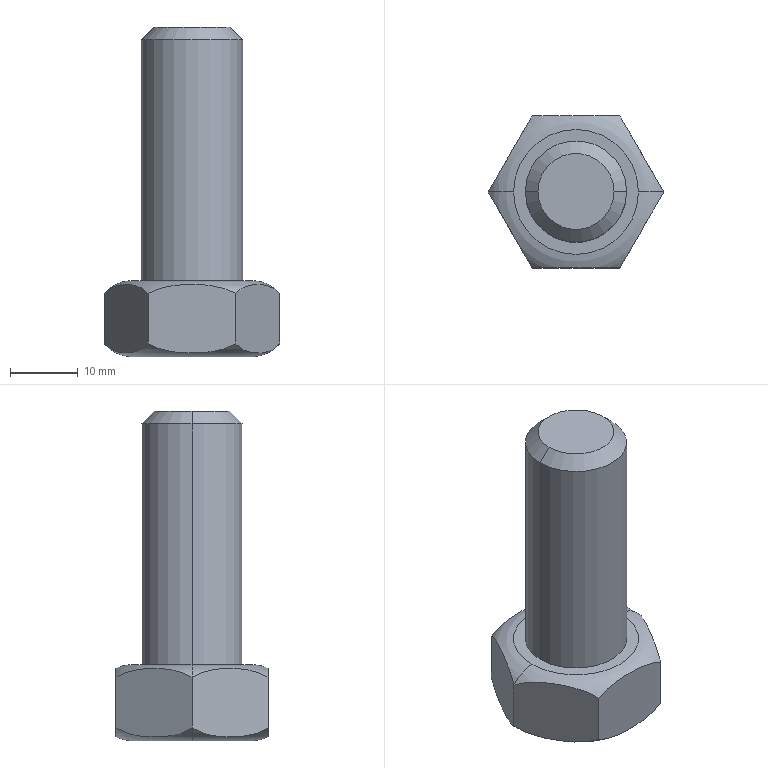Part | SolidWorks | features Chamfer 1, Extrusion 1, ICE 1, RevCut 1, Scale 1 | 1 solid | 17 faces | box 25.981 x 22.5 x 48.75 mm | volume 11356 mm3 | plane 9 | torus 4 | cone 2 | cylinder 2 | commonest cylinder face diameters 15 x2
STEP:
#1=CARTESIAN_POINT('',(9.24,0.00001748,-9.13));
#2=VERTEX_POINT('',#1);
#3=CARTESIAN_POINT('',(-9.24,0.00001748,-9.13));
#4=VERTEX_POINT('',#3);
#5=CARTESIAN_POINT('',(-0.000001168,0.00001748,-9.13));
#6=DIRECTION('',(0.,0.,1.));
#7=DIRECTION('',(1.,0.,0.));
#8=AXIS2_PLACEMENT_3D('',#5,#6,#7);
#9=CIRCLE('',#8,9.24);
#10=EDGE_CURVE('',#2,#4,#9,.T.);
#11=ORIENTED_EDGE('',*,*,#10,.T.);
#12=CARTESIAN_POINT('',(-12.99,0.00001748,-7.255));
#13=VERTEX_POINT('',#12);
#14=CARTESIAN_POINT('',(-8.781,0.00001748,-3.524));
#15=DIRECTION('',(0.,1.,0.));
#16=DIRECTION('',(-1.,0.,0.));
#17=AXIS2_PLACEMENT_3D('',#14,#15,#16);
#18=CIRCLE('',#17,5.625);
#19=EDGE_CURVE('',#4,#13,#18,.T.);
#20=ORIENTED_EDGE('',*,*,#19,.T.);
#21=CARTESIAN_POINT('',(-6.495,11.25,-7.255));
#22=VERTEX_POINT('',#21);
#23=CARTESIAN_POINT('',(-6.495,11.25,-7.255));
#24=CARTESIAN_POINT('',(-6.741,10.824,-7.533));
#25=CARTESIAN_POINT('',(-6.999,10.377,-7.746));
#26=CARTESIAN_POINT('',(-7.53,9.458,-8.089));
#27=CARTESIAN_POINT('',(-7.805,8.982,-8.217));
#28=CARTESIAN_POINT('',(-8.356,8.027,-8.41));
#29=CARTESIAN_POINT('',(-8.632,7.549,-8.474));
#30=CARTESIAN_POINT('',(-9.186,6.59,-8.558));
#31=CARTESIAN_POINT('',(-9.463,6.109,-8.578));
#32=CARTESIAN_POINT('',(-10.019,5.147,-8.578));
#33=CARTESIAN_POINT('',(-10.297,4.666,-8.559));
#34=CARTESIAN_POINT('',(-10.854,3.7,-8.474));
#35=CARTESIAN_POINT('',(-11.133,3.217,-8.409));
#36=CARTESIAN_POINT('',(-11.681,2.268,-8.217));
#37=CARTESIAN_POINT('',(-11.952,1.799,-8.091));
#38=CARTESIAN_POINT('',(-12.483,0.8793,-7.749));
#39=CARTESIAN_POINT('',(-12.745,0.4256,-7.532));
#40=CARTESIAN_POINT('',(-12.99,0.00001748,-7.255));
#41=B_SPLINE_CURVE_WITH_KNOTS('',3,(#23,#24,#25,#26,#27,#28,#29,#30,#31,#32,#33,#34,#35,#36,#37,#38,#39,#40),.UNSPECIFIED.,.F.,.F.,(4,2,2,2,2,2,2,2,4),(0.00000049,0.001672,0.003344,0.005016,0.006688,0.00836,0.01003,0.0117,0.01338),.UNSPECIFIED.);
#42=EDGE_CURVE('',#22,#13,#41,.T.);
#43=ORIENTED_EDGE('',*,*,#42,.F.);
#44=CARTESIAN_POINT('',(6.495,11.25,-7.255));
#45=VERTEX_POINT('',#44);
#46=CARTESIAN_POINT('',(6.495,11.25,-7.255));
#47=CARTESIAN_POINT('',(6.006,11.25,-7.531));
#48=CARTESIAN_POINT('',(5.491,11.25,-7.745));
#49=CARTESIAN_POINT('',(4.689,11.25,-8.004));
#50=CARTESIAN_POINT('',(4.417,11.25,-8.079));
#51=CARTESIAN_POINT('',(3.871,11.25,-8.21));
#52=CARTESIAN_POINT('',(3.597,11.25,-8.266));
#53=CARTESIAN_POINT('',(2.772,11.25,-8.41));
#54=CARTESIAN_POINT('',(2.218,11.25,-8.475));
#55=CARTESIAN_POINT('',(1.106,11.25,-8.559));
#56=CARTESIAN_POINT('',(0.5448,11.25,-8.579));
#57=CARTESIAN_POINT('',(-0.5739,11.25,-8.578));
#58=CARTESIAN_POINT('',(-1.13,11.25,-8.558));
#59=CARTESIAN_POINT('',(-2.235,11.25,-8.473));
#60=CARTESIAN_POINT('',(-2.784,11.25,-8.408));
#61=CARTESIAN_POINT('',(-3.872,11.25,-8.218));
#62=CARTESIAN_POINT('',(-4.412,11.25,-8.092));
#63=CARTESIAN_POINT('',(-5.476,11.25,-7.751));
#64=CARTESIAN_POINT('',(-6.004,11.25,-7.532));
#65=CARTESIAN_POINT('',(-6.495,11.25,-7.255));
#66=B_SPLINE_CURVE_WITH_KNOTS('',3,(#46,#47,#48,#49,#50,#51,#52,#53,#54,#55,#56,#57,#58,#59,#60,#61,#62,#63,#64,#65),.UNSPECIFIED.,.F.,.F.,(4,2,2,2,2,2,2,2,2,4),(0.03832,0.03997,0.0408,0.04163,0.04329,0.04495,0.0466,0.04826,0.04992,0.05157),.UNSPECIFIED.);
#67=EDGE_CURVE('',#45,#22,#66,.T.);
#68=ORIENTED_EDGE('',*,*,#67,.F.);
#69=CARTESIAN_POINT('',(12.99,0.00001748,-7.255));
#70=VERTEX_POINT('',#69);
#71=CARTESIAN_POINT('',(12.99,0.00001748,-7.255));
#72=CARTESIAN_POINT('',(12.744,0.4264,-7.533));
#73=CARTESIAN_POINT('',(12.486,0.8728,-7.746));
#74=CARTESIAN_POINT('',(11.956,1.792,-8.089));
#75=CARTESIAN_POINT('',(11.681,2.268,-8.217));
#76=CARTESIAN_POINT('',(11.13,3.223,-8.41));
#77=CARTESIAN_POINT('',(10.853,3.701,-8.474));
#78=CARTESIAN_POINT('',(10.3,4.66,-8.558));
#79=CARTESIAN_POINT('',(10.022,5.141,-8.578));
#80=CARTESIAN_POINT('',(9.467,6.103,-8.578));
#81=CARTESIAN_POINT('',(9.189,6.585,-8.559));
#82=CARTESIAN_POINT('',(8.631,7.55,-8.474));
#83=CARTESIAN_POINT('',(8.353,8.033,-8.409));
#84=CARTESIAN_POINT('',(7.804,8.982,-8.217));
#85=CARTESIAN_POINT('',(7.534,9.451,-8.091));
#86=CARTESIAN_POINT('',(7.003,10.371,-7.749));
#87=CARTESIAN_POINT('',(6.741,10.824,-7.532));
#88=CARTESIAN_POINT('',(6.495,11.25,-7.255));
#89=B_SPLINE_CURVE_WITH_KNOTS('',3,(#71,#72,#73,#74,#75,#76,#77,#78,#79,#80,#81,#82,#83,#84,#85,#86,#87,#88),.UNSPECIFIED.,.F.,.F.,(4,2,2,2,2,2,2,2,4),(0.00000049,0.001672,0.003344,0.005016,0.006688,0.00836,0.01003,0.0117,0.01338),.UNSPECIFIED.);
#90=EDGE_CURVE('',#70,#45,#89,.T.);
#91=ORIENTED_EDGE('',*,*,#90,.F.);
#92=CARTESIAN_POINT('',(8.781,0.00001748,-3.524));
#93=DIRECTION('',(0.,-1.,0.));
#94=DIRECTION('',(0.,0.,-1.));
#95=AXIS2_PLACEMENT_3D('',#92,#93,#94);
#96=CIRCLE('',#95,5.625);
#97=EDGE_CURVE('',#2,#70,#96,.T.);
#98=ORIENTED_EDGE('',*,*,#97,.F.);
#99=EDGE_LOOP('',(#11,#20,#43,#68,#91,#98));
#100=FACE_OUTER_BOUND('',#99,.T.);
#101=CARTESIAN_POINT('',(-0.000001168,0.00001748,-3.524));
#102=DIRECTION('',(0.,0.,1.));
#103=DIRECTION('',(1.,0.,0.));
#104=AXIS2_PLACEMENT_3D('',#101,#102,#103);
#105=TOROIDAL_SURFACE('',#104,8.781,5.625);
#106=ADVANCED_FACE('',(#100),#105,.T.);
#107=CARTESIAN_POINT('',(-12.99,0.00001748,0.2448));
#108=VERTEX_POINT('',#107);
#109=CARTESIAN_POINT('',(-6.495,11.25,0.2448));
#110=VERTEX_POINT('',#109);
#111=CARTESIAN_POINT('',(-12.99,0.00001748,0.2448));
#112=CARTESIAN_POINT('',(-12.744,0.4264,0.5225));
#113=CARTESIAN_POINT('',(-12.486,0.8728,0.736));
#114=CARTESIAN_POINT('',(-11.956,1.792,1.078));
#115=CARTESIAN_POINT('',(-11.681,2.268,1.207));
#116=CARTESIAN_POINT('',(-11.13,3.223,1.399));
#117=CARTESIAN_POINT('',(-10.853,3.701,1.464));
#118=CARTESIAN_POINT('',(-10.3,4.66,1.548));
#119=CARTESIAN_POINT('',(-10.022,5.141,1.568));
#120=CARTESIAN_POINT('',(-9.467,6.103,1.568));
#121=CARTESIAN_POINT('',(-9.189,6.585,1.548));
#122=CARTESIAN_POINT('',(-8.631,7.55,1.464));
#123=CARTESIAN_POINT('',(-8.353,8.033,1.398));
#124=CARTESIAN_POINT('',(-7.804,8.982,1.206));
#125=CARTESIAN_POINT('',(-7.534,9.451,1.08));
#126=CARTESIAN_POINT('',(-7.003,10.371,0.7389));
#127=CARTESIAN_POINT('',(-6.741,10.824,0.5219));
#128=CARTESIAN_POINT('',(-6.495,11.25,0.2448));
#129=B_SPLINE_CURVE_WITH_KNOTS('',3,(#111,#112,#113,#114,#115,#116,#117,#118,#119,#120,#121,#122,#123,#124,#125,#126,#127,#128),.UNSPECIFIED.,.F.,.F.,(4,2,2,2,2,2,2,2,4),(0.00000049,0.001672,0.003344,0.005016,0.006688,0.00836,0.01003,0.0117,0.01338),.UNSPECIFIED.);
#130=EDGE_CURVE('',#108,#110,#129,.T.);
#131=ORIENTED_EDGE('',*,*,#130,.F.);
#132=CARTESIAN_POINT('',(-9.24,0.00001748,2.12));
#133=VERTEX_POINT('',#132);
#134=CARTESIAN_POINT('',(-8.781,0.00001748,-3.486));
#135=DIRECTION('',(0.,1.,0.));
#136=DIRECTION('',(-1.,0.,0.));
#137=AXIS2_PLACEMENT_3D('',#134,#135,#136);
#138=CIRCLE('',#137,5.625);
#139=EDGE_CURVE('',#108,#133,#138,.T.);
#140=ORIENTED_EDGE('',*,*,#139,.T.);
#141=CARTESIAN_POINT('',(9.24,0.00001748,2.12));
#142=VERTEX_POINT('',#141);
#143=CARTESIAN_POINT('',(-0.000001168,0.00001748,2.12));
#144=DIRECTION('',(0.,0.,1.));
#145=DIRECTION('',(1.,0.,0.));
#146=AXIS2_PLACEMENT_3D('',#143,#144,#145);
#147=CIRCLE('',#146,9.24);
#148=EDGE_CURVE('',#142,#133,#147,.T.);
#149=ORIENTED_EDGE('',*,*,#148,.F.);
#150=CARTESIAN_POINT('',(12.99,0.00001748,0.2448));
#151=VERTEX_POINT('',#150);
#152=CARTESIAN_POINT('',(8.781,0.00001748,-3.486));
#153=DIRECTION('',(0.,-1.,0.));
#154=DIRECTION('',(0.,0.,-1.));
#155=AXIS2_PLACEMENT_3D('',#152,#153,#154);
#156=CIRCLE('',#155,5.625);
#157=EDGE_CURVE('',#151,#142,#156,.T.);
#158=ORIENTED_EDGE('',*,*,#157,.F.);
#159=CARTESIAN_POINT('',(6.495,11.25,0.2448));
#160=VERTEX_POINT('',#159);
#161=CARTESIAN_POINT('',(6.495,11.25,0.2448));
#162=CARTESIAN_POINT('',(6.741,10.824,0.5225));
#163=CARTESIAN_POINT('',(6.999,10.377,0.736));
#164=CARTESIAN_POINT('',(7.53,9.458,1.078));
#165=CARTESIAN_POINT('',(7.805,8.982,1.207));
#166=CARTESIAN_POINT('',(8.356,8.027,1.399));
#167=CARTESIAN_POINT('',(8.632,7.549,1.464));
#168=CARTESIAN_POINT('',(9.186,6.59,1.548));
#169=CARTESIAN_POINT('',(9.463,6.109,1.568));
#170=CARTESIAN_POINT('',(10.019,5.147,1.568));
#171=CARTESIAN_POINT('',(10.297,4.666,1.548));
#172=CARTESIAN_POINT('',(10.854,3.7,1.464));
#173=CARTESIAN_POINT('',(11.133,3.217,1.398));
#174=CARTESIAN_POINT('',(11.681,2.268,1.206));
#175=CARTESIAN_POINT('',(11.952,1.799,1.08));
#176=CARTESIAN_POINT('',(12.483,0.8793,0.7389));
#177=CARTESIAN_POINT('',(12.745,0.4256,0.5219));
#178=CARTESIAN_POINT('',(12.99,0.00001748,0.2448));
#179=B_SPLINE_CURVE_WITH_KNOTS('',3,(#161,#162,#163,#164,#165,#166,#167,#168,#169,#170,#171,#172,#173,#174,#175,#176,#177,#178),.UNSPECIFIED.,.F.,.F.,(4,2,2,2,2,2,2,2,4),(0.00000049,0.001672,0.003344,0.005016,0.006688,0.00836,0.01003,0.0117,0.01338),.UNSPECIFIED.);
#180=EDGE_CURVE('',#160,#151,#179,.T.);
#181=ORIENTED_EDGE('',*,*,#180,.F.);
#182=CARTESIAN_POINT('',(-6.495,11.25,0.2448));
#183=CARTESIAN_POINT('',(-6.006,11.25,0.5206));
#184=CARTESIAN_POINT('',(-5.491,11.25,0.735));
#185=CARTESIAN_POINT('',(-4.689,11.25,0.9932));
#186=CARTESIAN_POINT('',(-4.417,11.25,1.069));
#187=CARTESIAN_POINT('',(-3.871,11.25,1.2));
#188=CARTESIAN_POINT('',(-3.597,11.25,1.255));
#189=CARTESIAN_POINT('',(-2.772,11.25,1.399));
#190=CARTESIAN_POINT('',(-2.218,11.25,1.464));
#191=CARTESIAN_POINT('',(-1.106,11.25,1.548));
#192=CARTESIAN_POINT('',(-0.5448,11.25,1.568));
#193=CARTESIAN_POINT('',(0.5739,11.25,1.567));
#194=CARTESIAN_POINT('',(1.13,11.25,1.547));
#195=CARTESIAN_POINT('',(2.235,11.25,1.462));
#196=CARTESIAN_POINT('',(2.784,11.25,1.397));
#197=CARTESIAN_POINT('',(3.872,11.25,1.207));
#198=CARTESIAN_POINT('',(4.412,11.25,1.082));
#199=CARTESIAN_POINT('',(5.476,11.25,0.7405));
#200=CARTESIAN_POINT('',(6.004,11.25,0.5218));
#201=CARTESIAN_POINT('',(6.495,11.25,0.2448));
#202=B_SPLINE_CURVE_WITH_KNOTS('',3,(#182,#183,#184,#185,#186,#187,#188,#189,#190,#191,#192,#193,#194,#195,#196,#197,#198,#199,#200,#201),.UNSPECIFIED.,.F.,.F.,(4,2,2,2,2,2,2,2,2,4),(0.03832,0.03997,0.0408,0.04163,0.04329,0.04495,0.0466,0.04826,0.04992,0.05157),.UNSPECIFIED.);
#203=EDGE_CURVE('',#110,#160,#202,.T.);
#204=ORIENTED_EDGE('',*,*,#203,.F.);
#205=EDGE_LOOP('',(#131,#140,#149,#158,#181,#204));
#206=FACE_OUTER_BOUND('',#205,.T.);
#207=CARTESIAN_POINT('',(-0.000001168,0.00001748,-3.486));
#208=DIRECTION('',(0.,0.,1.));
#209=DIRECTION('',(1.,0.,0.));
#210=AXIS2_PLACEMENT_3D('',#207,#208,#209);
#211=TOROIDAL_SURFACE('',#210,8.781,5.625);
#212=ADVANCED_FACE('',(#206),#211,.T.);
#213=CARTESIAN_POINT('',(5.625,0.00001748,39.62));
#214=VERTEX_POINT('',#213);
#215=CARTESIAN_POINT('',(-5.625,0.00001748,39.62));
#216=VERTEX_POINT('',#215);
#217=CARTESIAN_POINT('',(-0.000001168,0.00001748,39.62));
#218=DIRECTION('',(0.,0.,1.));
#219=DIRECTION('',(1.,0.,0.));
#220=AXIS2_PLACEMENT_3D('',#217,#218,#219);
#221=CIRCLE('',#220,5.625);
#222=EDGE_CURVE('',#214,#216,#221,.T.);
#223=ORIENTED_EDGE('',*,*,#222,.F.);
#224=CARTESIAN_POINT('',(7.5,0.00001748,37.745));
#225=VERTEX_POINT('',#224);
#226=CARTESIAN_POINT('',(5.625,0.00001748,39.62));
#227=DIRECTION('',(0.7071,0.,-0.7071));
#228=VECTOR('',#227,1000.);
#229=LINE('',#226,#228);
#230=EDGE_CURVE('',#214,#225,#229,.T.);
#231=ORIENTED_EDGE('',*,*,#230,.T.);
#232=CARTESIAN_POINT('',(-7.5,0.00001748,37.745));
#233=VERTEX_POINT('',#232);
#234=CARTESIAN_POINT('',(-0.000001168,0.00001748,37.745));
#235=DIRECTION('',(0.,0.,-1.));
#236=DIRECTION('',(1.,0.,0.));
#237=AXIS2_PLACEMENT_3D('',#234,#235,#236);
#238=CIRCLE('',#237,7.5);
#239=EDGE_CURVE('',#233,#225,#238,.T.);
#240=ORIENTED_EDGE('',*,*,#239,.F.);
#241=CARTESIAN_POINT('',(-5.625,0.00001748,39.62));
#242=DIRECTION('',(-0.7071,0.,-0.7071));
#243=VECTOR('',#242,1000.);
#244=LINE('',#241,#243);
#245=EDGE_CURVE('',#216,#233,#244,.T.);
#246=ORIENTED_EDGE('',*,*,#245,.F.);
#247=EDGE_LOOP('',(#223,#231,#240,#246));
#248=FACE_OUTER_BOUND('',#247,.T.);
#249=CARTESIAN_POINT('',(-0.000001168,0.00001748,39.62));
#250=DIRECTION('',(0.,0.,-1.));
#251=DIRECTION('',(-1.,0.,0.));
#252=AXIS2_PLACEMENT_3D('',#249,#250,#251);
#253=CONICAL_SURFACE('',#252,5.625,0.7854);
#254=ADVANCED_FACE('',(#248),#253,.T.);
#255=ORIENTED_EDGE('',*,*,#239,.T.);
#256=CARTESIAN_POINT('',(7.5,0.00001748,2.12));
#257=VERTEX_POINT('',#256);
#258=CARTESIAN_POINT('',(7.5,0.00001748,39.62));
#259=DIRECTION('',(0.,0.,-1.));
#260=VECTOR('',#259,1000.);
#261=LINE('',#258,#260);
#262=EDGE_CURVE('',#225,#257,#261,.T.);
#263=ORIENTED_EDGE('',*,*,#262,.T.);
#264=CARTESIAN_POINT('',(-7.5,0.00001748,2.12));
#265=VERTEX_POINT('',#264);
#266=CARTESIAN_POINT('',(-0.000001168,0.00001748,2.12));
#267=DIRECTION('',(0.,0.,1.));
#268=DIRECTION('',(1.,0.,0.));
#269=AXIS2_PLACEMENT_3D('',#266,#267,#268);
#270=CIRCLE('',#269,7.5);
#271=EDGE_CURVE('',#257,#265,#270,.T.);
#272=ORIENTED_EDGE('',*,*,#271,.T.);
#273=CARTESIAN_POINT('',(-7.5,0.00001748,39.62));
#274=DIRECTION('',(0.,0.,-1.));
#275=VECTOR('',#274,1000.);
#276=LINE('',#273,#275);
#277=EDGE_CURVE('',#233,#265,#276,.T.);
#278=ORIENTED_EDGE('',*,*,#277,.F.);
#279=EDGE_LOOP('',(#255,#263,#272,#278));
#280=FACE_OUTER_BOUND('',#279,.T.);
#281=CARTESIAN_POINT('',(-0.000001168,0.00001748,39.62));
#282=DIRECTION('',(0.,0.,-1.));
#283=DIRECTION('',(-1.,0.,0.));
#284=AXIS2_PLACEMENT_3D('',#281,#282,#283);
#285=CYLINDRICAL_SURFACE('',#284,7.5);
#286=ADVANCED_FACE('',(#280),#285,.T.);
#287=CARTESIAN_POINT('',(-0.000001168,0.00001748,2.12));
#288=DIRECTION('',(0.,0.,1.));
#289=DIRECTION('',(1.,0.,0.));
#290=AXIS2_PLACEMENT_3D('',#287,#288,#289);
#291=CIRCLE('',#290,7.5);
#292=EDGE_CURVE('',#265,#257,#291,.T.);
#293=ORIENTED_EDGE('',*,*,#292,.F.);
#294=ORIENTED_EDGE('',*,*,#271,.F.);
#295=EDGE_LOOP('',(#293,#294));
#296=FACE_BOUND('',#295,.T.);
#297=ORIENTED_EDGE('',*,*,#148,.T.);
#298=CARTESIAN_POINT('',(-0.000001168,0.00001748,2.12));
#299=DIRECTION('',(0.,0.,1.));
#300=DIRECTION('',(1.,0.,0.));
#301=AXIS2_PLACEMENT_3D('',#298,#299,#300);
#302=CIRCLE('',#301,9.24);
#303=EDGE_CURVE('',#133,#142,#302,.T.);
#304=ORIENTED_EDGE('',*,*,#303,.T.);
#305=EDGE_LOOP('',(#297,#304));
#306=FACE_OUTER_BOUND('',#305,.T.);
#307=CARTESIAN_POINT('',(-0.000001168,0.00001748,2.12));
#308=DIRECTION('',(0.,0.,1.));
#309=DIRECTION('',(1.,0.,0.));
#310=AXIS2_PLACEMENT_3D('',#307,#308,#309);
#311=PLANE('',#310);
#312=ADVANCED_FACE('',(#296,#306),#311,.T.);
#313=ORIENTED_EDGE('',*,*,#262,.F.);
#314=CARTESIAN_POINT('',(-0.000001168,0.00001748,37.745));
#315=DIRECTION('',(0.,0.,-1.));
#316=DIRECTION('',(1.,0.,0.));
#317=AXIS2_PLACEMENT_3D('',#314,#315,#316);
#318=CIRCLE('',#317,7.5);
#319=EDGE_CURVE('',#225,#233,#318,.T.);
#320=ORIENTED_EDGE('',*,*,#319,.T.);
#321=ORIENTED_EDGE('',*,*,#277,.T.);
#322=ORIENTED_EDGE('',*,*,#292,.T.);
#323=EDGE_LOOP('',(#313,#320,#321,#322));
#324=FACE_OUTER_BOUND('',#323,.T.);
#325=CARTESIAN_POINT('',(-0.000001168,0.00001748,39.62));
#326=DIRECTION('',(0.,0.,-1.));
#327=DIRECTION('',(-1.,0.,0.));
#328=AXIS2_PLACEMENT_3D('',#325,#326,#327);
#329=CYLINDRICAL_SURFACE('',#328,7.5);
#330=ADVANCED_FACE('',(#324),#329,.T.);
#331=CARTESIAN_POINT('',(-0.000001168,0.00001748,39.62));
#332=DIRECTION('',(0.,0.,1.));
#333=DIRECTION('',(1.,0.,0.));
#334=AXIS2_PLACEMENT_3D('',#331,#332,#333);
#335=CIRCLE('',#334,5.625);
#336=EDGE_CURVE('',#216,#214,#335,.T.);
#337=ORIENTED_EDGE('',*,*,#336,.T.);
#338=ORIENTED_EDGE('',*,*,#222,.T.);
#339=EDGE_LOOP('',(#337,#338));
#340=FACE_OUTER_BOUND('',#339,.T.);
#341=CARTESIAN_POINT('',(-0.000001168,0.00001748,39.62));
#342=DIRECTION('',(0.,0.,1.));
#343=DIRECTION('',(1.,0.,0.));
#344=AXIS2_PLACEMENT_3D('',#341,#342,#343);
#345=PLANE('',#344);
#346=ADVANCED_FACE('',(#340),#345,.T.);
#347=ORIENTED_EDGE('',*,*,#230,.F.);
#348=ORIENTED_EDGE('',*,*,#336,.F.);
#349=ORIENTED_EDGE('',*,*,#245,.T.);
#350=ORIENTED_EDGE('',*,*,#319,.F.);
#351=EDGE_LOOP('',(#347,#348,#349,#350));
#352=FACE_OUTER_BOUND('',#351,.T.);
#353=CARTESIAN_POINT('',(-0.000001168,0.00001748,39.62));
#354=DIRECTION('',(0.,0.,-1.));
#355=DIRECTION('',(-1.,0.,0.));
#356=AXIS2_PLACEMENT_3D('',#353,#354,#355);
#357=CONICAL_SURFACE('',#356,5.625,0.7854);
#358=ADVANCED_FACE('',(#352),#357,.T.);
#359=ORIENTED_EDGE('',*,*,#139,.F.);
#360=CARTESIAN_POINT('',(-6.495,-11.25,0.2448));
#361=VERTEX_POINT('',#360);
#362=CARTESIAN_POINT('',(-6.495,-11.25,0.2448));
#363=CARTESIAN_POINT('',(-6.741,-10.824,0.5225));
#364=CARTESIAN_POINT('',(-6.999,-10.377,0.736));
#365=CARTESIAN_POINT('',(-7.53,-9.458,1.078));
#366=CARTESIAN_POINT('',(-7.805,-8.982,1.207));
#367=CARTESIAN_POINT('',(-8.356,-8.027,1.399));
#368=CARTESIAN_POINT('',(-8.632,-7.549,1.464));
#369=CARTESIAN_POINT('',(-9.186,-6.59,1.548));
#370=CARTESIAN_POINT('',(-9.463,-6.109,1.568));
#371=CARTESIAN_POINT('',(-10.019,-5.147,1.568));
#372=CARTESIAN_POINT('',(-10.297,-4.665,1.548));
#373=CARTESIAN_POINT('',(-10.854,-3.7,1.464));
#374=CARTESIAN_POINT('',(-11.133,-3.217,1.398));
#375=CARTESIAN_POINT('',(-11.681,-2.268,1.206));
#376=CARTESIAN_POINT('',(-11.952,-1.799,1.08));
#377=CARTESIAN_POINT('',(-12.483,-0.8793,0.7389));
#378=CARTESIAN_POINT('',(-12.745,-0.4255,0.5219));
#379=CARTESIAN_POINT('',(-12.99,0.00001748,0.2448));
#380=B_SPLINE_CURVE_WITH_KNOTS('',3,(#362,#363,#364,#365,#366,#367,#368,#369,#370,#371,#372,#373,#374,#375,#376,#377,#378,#379),.UNSPECIFIED.,.F.,.F.,(4,2,2,2,2,2,2,2,4),(0.00000049,0.001672,0.003344,0.005016,0.006688,0.00836,0.01003,0.0117,0.01338),.UNSPECIFIED.);
#381=EDGE_CURVE('',#361,#108,#380,.T.);
#382=ORIENTED_EDGE('',*,*,#381,.F.);
#383=CARTESIAN_POINT('',(6.495,-11.25,0.2448));
#384=VERTEX_POINT('',#383);
#385=CARTESIAN_POINT('',(6.495,-11.25,0.2448));
#386=CARTESIAN_POINT('',(6.006,-11.25,0.5206));
#387=CARTESIAN_POINT('',(5.491,-11.25,0.735));
#388=CARTESIAN_POINT('',(4.689,-11.25,0.9932));
#389=CARTESIAN_POINT('',(4.417,-11.25,1.069));
#390=CARTESIAN_POINT('',(3.871,-11.25,1.2));
#391=CARTESIAN_POINT('',(3.597,-11.25,1.255));
#392=CARTESIAN_POINT('',(2.772,-11.25,1.399));
#393=CARTESIAN_POINT('',(2.218,-11.25,1.464));
#394=CARTESIAN_POINT('',(1.106,-11.25,1.548));
#395=CARTESIAN_POINT('',(0.5448,-11.25,1.568));
#396=CARTESIAN_POINT('',(-0.5739,-11.25,1.567));
#397=CARTESIAN_POINT('',(-1.13,-11.25,1.547));
#398=CARTESIAN_POINT('',(-2.235,-11.25,1.462));
#399=CARTESIAN_POINT('',(-2.784,-11.25,1.397));
#400=CARTESIAN_POINT('',(-3.872,-11.25,1.207));
#401=CARTESIAN_POINT('',(-4.412,-11.25,1.082));
#402=CARTESIAN_POINT('',(-5.476,-11.25,0.7405));
#403=CARTESIAN_POINT('',(-6.004,-11.25,0.5218));
#404=CARTESIAN_POINT('',(-6.495,-11.25,0.2448));
#405=B_SPLINE_CURVE_WITH_KNOTS('',3,(#385,#386,#387,#388,#389,#390,#391,#392,#393,#394,#395,#396,#397,#398,#399,#400,#401,#402,#403,#404),.UNSPECIFIED.,.F.,.F.,(4,2,2,2,2,2,2,2,2,4),(0.03832,0.03997,0.0408,0.04163,0.04329,0.04495,0.0466,0.04826,0.04992,0.05157),.UNSPECIFIED.);
#406=EDGE_CURVE('',#384,#361,#405,.T.);
#407=ORIENTED_EDGE('',*,*,#406,.F.);
#408=CARTESIAN_POINT('',(12.99,0.00001748,0.2448));
#409=CARTESIAN_POINT('',(12.744,-0.4264,0.5225));
#410=CARTESIAN_POINT('',(12.486,-0.8728,0.736));
#411=CARTESIAN_POINT('',(11.956,-1.792,1.078));
#412=CARTESIAN_POINT('',(11.681,-2.268,1.207));
#413=CARTESIAN_POINT('',(11.13,-3.223,1.399));
#414=CARTESIAN_POINT('',(10.853,-3.701,1.464));
#415=CARTESIAN_POINT('',(10.3,-4.66,1.548));
#416=CARTESIAN_POINT('',(10.022,-5.141,1.568));
#417=CARTESIAN_POINT('',(9.467,-6.103,1.568));
#418=CARTESIAN_POINT('',(9.189,-6.584,1.548));
#419=CARTESIAN_POINT('',(8.631,-7.55,1.464));
#420=CARTESIAN_POINT('',(8.353,-8.033,1.398));
#421=CARTESIAN_POINT('',(7.804,-8.982,1.206));
#422=CARTESIAN_POINT('',(7.534,-9.451,1.08));
#423=CARTESIAN_POINT('',(7.003,-10.371,0.7389));
#424=CARTESIAN_POINT('',(6.741,-10.824,0.5219));
#425=CARTESIAN_POINT('',(6.495,-11.25,0.2448));
#426=B_SPLINE_CURVE_WITH_KNOTS('',3,(#408,#409,#410,#411,#412,#413,#414,#415,#416,#417,#418,#419,#420,#421,#422,#423,#424,#425),.UNSPECIFIED.,.F.,.F.,(4,2,2,2,2,2,2,2,4),(0.00000049,0.001672,0.003344,0.005016,0.006688,0.00836,0.01003,0.0117,0.01338),.UNSPECIFIED.);
#427=EDGE_CURVE('',#151,#384,#426,.T.);
#428=ORIENTED_EDGE('',*,*,#427,.F.);
#429=ORIENTED_EDGE('',*,*,#157,.T.);
#430=ORIENTED_EDGE('',*,*,#303,.F.);
#431=EDGE_LOOP('',(#359,#382,#407,#428,#429,#430));
#432=FACE_OUTER_BOUND('',#431,.T.);
#433=CARTESIAN_POINT('',(-0.000001168,0.00001748,-3.486));
#434=DIRECTION('',(0.,0.,1.));
#435=DIRECTION('',(1.,0.,0.));
#436=AXIS2_PLACEMENT_3D('',#433,#434,#435);
#437=TOROIDAL_SURFACE('',#436,8.781,5.625);
#438=ADVANCED_FACE('',(#432),#437,.T.);
#439=ORIENTED_EDGE('',*,*,#10,.F.);
#440=CARTESIAN_POINT('',(-0.000001168,0.00001748,-9.13));
#441=DIRECTION('',(0.,0.,1.));
#442=DIRECTION('',(1.,0.,0.));
#443=AXIS2_PLACEMENT_3D('',#440,#441,#442);
#444=CIRCLE('',#443,9.24);
#445=EDGE_CURVE('',#4,#2,#444,.T.);
#446=ORIENTED_EDGE('',*,*,#445,.F.);
#447=EDGE_LOOP('',(#439,#446));
#448=FACE_OUTER_BOUND('',#447,.T.);
#449=CARTESIAN_POINT('',(-0.000001168,0.00001748,-9.13));
#450=DIRECTION('',(0.,0.,1.));
#451=DIRECTION('',(1.,0.,0.));
#452=AXIS2_PLACEMENT_3D('',#449,#450,#451);
#453=PLANE('',#452);
#454=ADVANCED_FACE('',(#448),#453,.F.);
#455=ORIENTED_EDGE('',*,*,#19,.F.);
#456=ORIENTED_EDGE('',*,*,#445,.T.);
#457=ORIENTED_EDGE('',*,*,#97,.T.);
#458=CARTESIAN_POINT('',(6.495,-11.25,-7.255));
#459=VERTEX_POINT('',#458);
#460=CARTESIAN_POINT('',(6.495,-11.25,-7.255));
#461=CARTESIAN_POINT('',(6.741,-10.824,-7.533));
#462=CARTESIAN_POINT('',(6.999,-10.377,-7.746));
#463=CARTESIAN_POINT('',(7.53,-9.458,-8.089));
#464=CARTESIAN_POINT('',(7.805,-8.982,-8.217));
#465=CARTESIAN_POINT('',(8.356,-8.027,-8.41));
#466=CARTESIAN_POINT('',(8.632,-7.549,-8.474));
#467=CARTESIAN_POINT('',(9.186,-6.59,-8.558));
#468=CARTESIAN_POINT('',(9.463,-6.109,-8.578));
#469=CARTESIAN_POINT('',(10.019,-5.147,-8.578));
#470=CARTESIAN_POINT('',(10.297,-4.665,-8.559));
#471=CARTESIAN_POINT('',(10.854,-3.7,-8.474));
#472=CARTESIAN_POINT('',(11.133,-3.217,-8.409));
#473=CARTESIAN_POINT('',(11.681,-2.268,-8.217));
#474=CARTESIAN_POINT('',(11.952,-1.799,-8.091));
#475=CARTESIAN_POINT('',(12.483,-0.8793,-7.749));
#476=CARTESIAN_POINT('',(12.745,-0.4255,-7.532));
#477=CARTESIAN_POINT('',(12.99,0.00001748,-7.255));
#478=B_SPLINE_CURVE_WITH_KNOTS('',3,(#460,#461,#462,#463,#464,#465,#466,#467,#468,#469,#470,#471,#472,#473,#474,#475,#476,#477),.UNSPECIFIED.,.F.,.F.,(4,2,2,2,2,2,2,2,4),(0.00000049,0.001672,0.003344,0.005016,0.006688,0.00836,0.01003,0.0117,0.01338),.UNSPECIFIED.);
#479=EDGE_CURVE('',#459,#70,#478,.T.);
#480=ORIENTED_EDGE('',*,*,#479,.F.);
#481=CARTESIAN_POINT('',(-6.495,-11.25,-7.255));
#482=VERTEX_POINT('',#481);
#483=CARTESIAN_POINT('',(-6.495,-11.25,-7.255));
#484=CARTESIAN_POINT('',(-6.006,-11.25,-7.531));
#485=CARTESIAN_POINT('',(-5.491,-11.25,-7.745));
#486=CARTESIAN_POINT('',(-4.689,-11.25,-8.004));
#487=CARTESIAN_POINT('',(-4.417,-11.25,-8.079));
#488=CARTESIAN_POINT('',(-3.871,-11.25,-8.21));
#489=CARTESIAN_POINT('',(-3.597,-11.25,-8.266));
#490=CARTESIAN_POINT('',(-2.772,-11.25,-8.41));
#491=CARTESIAN_POINT('',(-2.218,-11.25,-8.475));
#492=CARTESIAN_POINT('',(-1.106,-11.25,-8.559));
#493=CARTESIAN_POINT('',(-0.5448,-11.25,-8.579));
#494=CARTESIAN_POINT('',(0.5739,-11.25,-8.578));
#495=CARTESIAN_POINT('',(1.13,-11.25,-8.558));
#496=CARTESIAN_POINT('',(2.235,-11.25,-8.473));
#497=CARTESIAN_POINT('',(2.784,-11.25,-8.408));
#498=CARTESIAN_POINT('',(3.872,-11.25,-8.218));
#499=CARTESIAN_POINT('',(4.412,-11.25,-8.092));
#500=CARTESIAN_POINT('',(5.476,-11.25,-7.751));
#501=CARTESIAN_POINT('',(6.004,-11.25,-7.532));
#502=CARTESIAN_POINT('',(6.495,-11.25,-7.255));
#503=B_SPLINE_CURVE_WITH_KNOTS('',3,(#483,#484,#485,#486,#487,#488,#489,#490,#491,#492,#493,#494,#495,#496,#497,#498,#499,#500,#501,#502),.UNSPECIFIED.,.F.,.F.,(4,2,2,2,2,2,2,2,2,4),(0.03832,0.03997,0.0408,0.04163,0.04329,0.04495,0.0466,0.04826,0.04992,0.05157),.UNSPECIFIED.);
#504=EDGE_CURVE('',#482,#459,#503,.T.);
#505=ORIENTED_EDGE('',*,*,#504,.F.);
#506=CARTESIAN_POINT('',(-12.99,0.00001748,-7.255));
#507=CARTESIAN_POINT('',(-12.744,-0.4264,-7.533));
#508=CARTESIAN_POINT('',(-12.486,-0.8728,-7.746));
#509=CARTESIAN_POINT('',(-11.956,-1.792,-8.089));
#510=CARTESIAN_POINT('',(-11.681,-2.268,-8.217));
#511=CARTESIAN_POINT('',(-11.13,-3.223,-8.41));
#512=CARTESIAN_POINT('',(-10.853,-3.701,-8.474));
#513=CARTESIAN_POINT('',(-10.3,-4.66,-8.558));
#514=CARTESIAN_POINT('',(-10.022,-5.141,-8.578));
#515=CARTESIAN_POINT('',(-9.467,-6.103,-8.578));
#516=CARTESIAN_POINT('',(-9.189,-6.584,-8.559));
#517=CARTESIAN_POINT('',(-8.631,-7.55,-8.474));
#518=CARTESIAN_POINT('',(-8.353,-8.033,-8.409));
#519=CARTESIAN_POINT('',(-7.804,-8.982,-8.217));
#520=CARTESIAN_POINT('',(-7.534,-9.451,-8.091));
#521=CARTESIAN_POINT('',(-7.003,-10.371,-7.749));
#522=CARTESIAN_POINT('',(-6.741,-10.824,-7.532));
#523=CARTESIAN_POINT('',(-6.495,-11.25,-7.255));
#524=B_SPLINE_CURVE_WITH_KNOTS('',3,(#506,#507,#508,#509,#510,#511,#512,#513,#514,#515,#516,#517,#518,#519,#520,#521,#522,#523),.UNSPECIFIED.,.F.,.F.,(4,2,2,2,2,2,2,2,4),(0.00000049,0.001672,0.003344,0.005016,0.006688,0.00836,0.01003,0.0117,0.01338),.UNSPECIFIED.);
#525=EDGE_CURVE('',#13,#482,#524,.T.);
#526=ORIENTED_EDGE('',*,*,#525,.F.);
#527=EDGE_LOOP('',(#455,#456,#457,#480,#505,#526));
#528=FACE_OUTER_BOUND('',#527,.T.);
#529=CARTESIAN_POINT('',(-0.000001168,0.00001748,-3.524));
#530=DIRECTION('',(0.,0.,1.));
#531=DIRECTION('',(1.,0.,0.));
#532=AXIS2_PLACEMENT_3D('',#529,#530,#531);
#533=TOROIDAL_SURFACE('',#532,8.781,5.625);
#534=ADVANCED_FACE('',(#528),#533,.T.);
#535=CARTESIAN_POINT('',(6.495,-11.25,2.12));
#536=DIRECTION('',(0.,0.,-1.));
#537=VECTOR('',#536,1000.);
#538=LINE('',#535,#537);
#539=EDGE_CURVE('',#384,#459,#538,.T.);
#540=ORIENTED_EDGE('',*,*,#539,.F.);
#541=ORIENTED_EDGE('',*,*,#406,.T.);
#542=CARTESIAN_POINT('',(-6.495,-11.25,2.12));
#543=DIRECTION('',(0.,0.,-1.));
#544=VECTOR('',#543,1000.);
#545=LINE('',#542,#544);
#546=EDGE_CURVE('',#361,#482,#545,.T.);
#547=ORIENTED_EDGE('',*,*,#546,.T.);
#548=ORIENTED_EDGE('',*,*,#504,.T.);
#549=EDGE_LOOP('',(#540,#541,#547,#548));
#550=FACE_OUTER_BOUND('',#549,.T.);
#551=CARTESIAN_POINT('',(-6.495,-11.25,2.12));
#552=DIRECTION('',(0.,1.,0.));
#553=DIRECTION('',(-1.,0.,0.));
#554=AXIS2_PLACEMENT_3D('',#551,#552,#553);
#555=PLANE('',#554);
#556=ADVANCED_FACE('',(#550),#555,.F.);
#557=ORIENTED_EDGE('',*,*,#546,.F.);
#558=ORIENTED_EDGE('',*,*,#381,.T.);
#559=CARTESIAN_POINT('',(-12.99,0.00001748,2.12));
#560=DIRECTION('',(0.,0.,-1.));
#561=VECTOR('',#560,1000.);
#562=LINE('',#559,#561);
#563=EDGE_CURVE('',#108,#13,#562,.T.);
#564=ORIENTED_EDGE('',*,*,#563,.T.);
#565=ORIENTED_EDGE('',*,*,#525,.T.);
#566=EDGE_LOOP('',(#557,#558,#564,#565));
#567=FACE_OUTER_BOUND('',#566,.T.);
#568=CARTESIAN_POINT('',(-12.99,0.00001748,2.12));
#569=DIRECTION('',(0.866,0.5,0.));
#570=DIRECTION('',(-0.5,0.866,0.));
#571=AXIS2_PLACEMENT_3D('',#568,#569,#570);
#572=PLANE('',#571);
#573=ADVANCED_FACE('',(#567),#572,.F.);
#574=ORIENTED_EDGE('',*,*,#563,.F.);
#575=ORIENTED_EDGE('',*,*,#130,.T.);
#576=CARTESIAN_POINT('',(-6.495,11.25,2.12));
#577=DIRECTION('',(0.,0.,-1.));
#578=VECTOR('',#577,1000.);
#579=LINE('',#576,#578);
#580=EDGE_CURVE('',#110,#22,#579,.T.);
#581=ORIENTED_EDGE('',*,*,#580,.T.);
#582=ORIENTED_EDGE('',*,*,#42,.T.);
#583=EDGE_LOOP('',(#574,#575,#581,#582));
#584=FACE_OUTER_BOUND('',#583,.T.);
#585=CARTESIAN_POINT('',(-6.495,11.25,2.12));
#586=DIRECTION('',(0.866,-0.5,0.));
#587=DIRECTION('',(0.5,0.866,0.));
#588=AXIS2_PLACEMENT_3D('',#585,#586,#587);
#589=PLANE('',#588);
#590=ADVANCED_FACE('',(#584),#589,.F.);
#591=ORIENTED_EDGE('',*,*,#580,.F.);
#592=ORIENTED_EDGE('',*,*,#203,.T.);
#593=CARTESIAN_POINT('',(6.495,11.25,2.12));
#594=DIRECTION('',(0.,0.,-1.));
#595=VECTOR('',#594,1000.);
#596=LINE('',#593,#595);
#597=EDGE_CURVE('',#160,#45,#596,.T.);
#598=ORIENTED_EDGE('',*,*,#597,.T.);
#599=ORIENTED_EDGE('',*,*,#67,.T.);
#600=EDGE_LOOP('',(#591,#592,#598,#599));
#601=FACE_OUTER_BOUND('',#600,.T.);
#602=CARTESIAN_POINT('',(6.495,11.25,2.12));
#603=DIRECTION('',(0.,-1.,0.));
#604=DIRECTION('',(0.,0.,-1.));
#605=AXIS2_PLACEMENT_3D('',#602,#603,#604);
#606=PLANE('',#605);
#607=ADVANCED_FACE('',(#601),#606,.F.);
#608=ORIENTED_EDGE('',*,*,#597,.F.);
#609=ORIENTED_EDGE('',*,*,#180,.T.);
#610=CARTESIAN_POINT('',(12.99,0.00001748,2.12));
#611=DIRECTION('',(0.,0.,-1.));
#612=VECTOR('',#611,1000.);
#613=LINE('',#610,#612);
#614=EDGE_CURVE('',#151,#70,#613,.T.);
#615=ORIENTED_EDGE('',*,*,#614,.T.);
#616=ORIENTED_EDGE('',*,*,#90,.T.);
#617=EDGE_LOOP('',(#608,#609,#615,#616));
#618=FACE_OUTER_BOUND('',#617,.T.);
#619=CARTESIAN_POINT('',(12.99,0.00001748,2.12));
#620=DIRECTION('',(-0.866,-0.5,0.));
#621=DIRECTION('',(0.5,-0.866,0.));
#622=AXIS2_PLACEMENT_3D('',#619,#620,#621);
#623=PLANE('',#622);
#624=ADVANCED_FACE('',(#618),#623,.F.);
#625=ORIENTED_EDGE('',*,*,#614,.F.);
#626=ORIENTED_EDGE('',*,*,#427,.T.);
#627=ORIENTED_EDGE('',*,*,#539,.T.);
#628=ORIENTED_EDGE('',*,*,#479,.T.);
#629=EDGE_LOOP('',(#625,#626,#627,#628));
#630=FACE_OUTER_BOUND('',#629,.T.);
#631=CARTESIAN_POINT('',(6.495,-11.25,2.12));
#632=DIRECTION('',(-0.866,0.5,0.));
#633=DIRECTION('',(-0.5,-0.866,0.));
#634=AXIS2_PLACEMENT_3D('',#631,#632,#633);
#635=PLANE('',#634);
#636=ADVANCED_FACE('',(#630),#635,.F.);
#637=CLOSED_SHELL('',(#106,#212,#254,#286,#312,#330,#346,#358,#438,#454,#534,#556,#573,#590,#607,#624,#636));
#638=MANIFOLD_SOLID_BREP('',#637);
#639=CARTESIAN_POINT('',(0.,0.,0.));
#640=DIRECTION('',(0.,0.,1.));
#641=DIRECTION('',(1.,0.,0.));
#642=AXIS2_PLACEMENT_3D('',#639,#640,#641);
#643=(LENGTH_UNIT()NAMED_UNIT(*)SI_UNIT(.MILLI.,.METRE.));
#644=UNCERTAINTY_MEASURE_WITH_UNIT(LENGTH_MEASURE(0.00001),#643,'','');
#645=(NAMED_UNIT(*)PLANE_ANGLE_UNIT()SI_UNIT($,.RADIAN.));
#646=(NAMED_UNIT(*)SI_UNIT($,.STERADIAN.)SOLID_ANGLE_UNIT());
#647=(GEOMETRIC_REPRESENTATION_CONTEXT(3)GLOBAL_UNCERTAINTY_ASSIGNED_CONTEXT((#644))GLOBAL_UNIT_ASSIGNED_CONTEXT((#643,#645,#646))REPRESENTATION_CONTEXT('',''));
#648=ADVANCED_BREP_SHAPE_REPRESENTATION('',(#638,#642),#647);